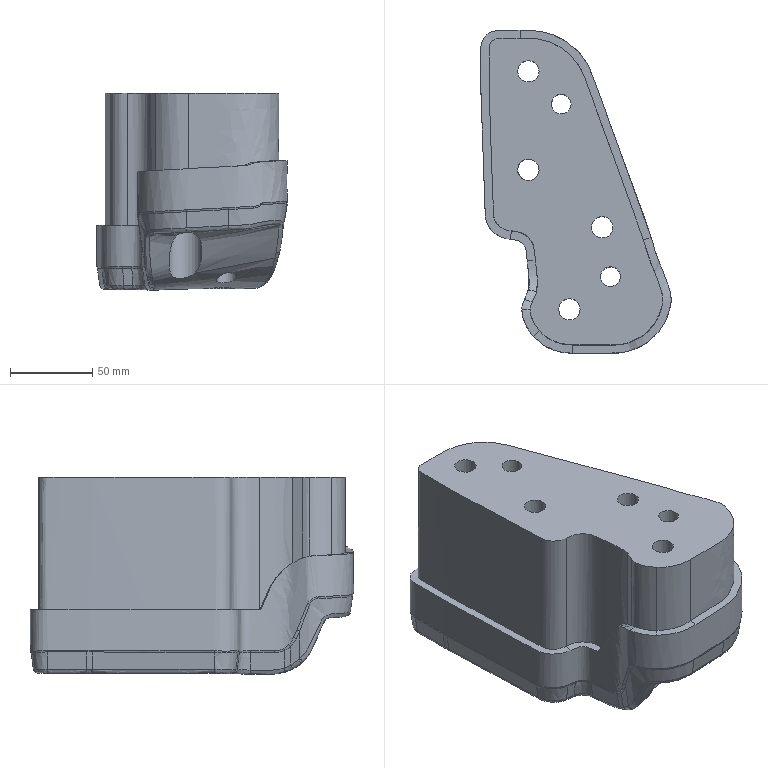Part | NX | features solid 2 | 1 solid | 115 faces | box 115.983 x 196.779 x 120.222 mm | volume 1406747 mm3 | spline 95 | plane 10 | cylinder 10 | commonest cylinder face diameters 13 x4 20 x4 12 x2